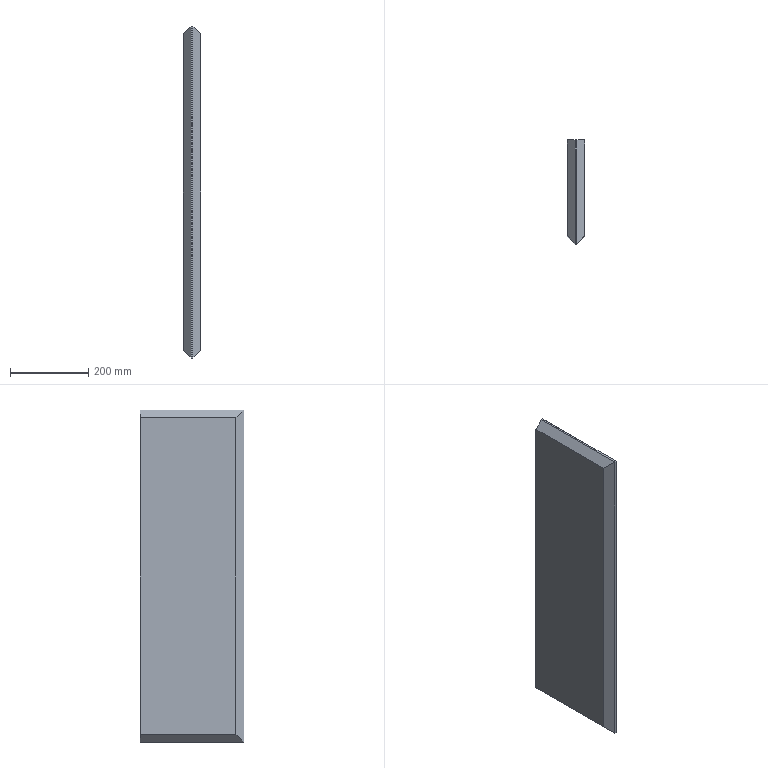Part | SolidWorks | features Chamfer 1, Extrusion 1 | 1 solid | 12 faces | box 45 x 265 x 850 mm | volume 9594917 mm3 | plane 12
STEP:
#1=CARTESIAN_POINT('',(2.5,132.5,425.));
#2=VERTEX_POINT('',#1);
#3=CARTESIAN_POINT('',(-2.5,132.5,425.));
#4=VERTEX_POINT('',#3);
#5=CARTESIAN_POINT('',(22.5,132.5,425.));
#6=DIRECTION('',(-1.,0.,0.));
#7=VECTOR('',#6,1000.);
#8=LINE('',#5,#7);
#9=EDGE_CURVE('',#2,#4,#8,.T.);
#10=ORIENTED_EDGE('',*,*,#9,.T.);
#11=CARTESIAN_POINT('',(-2.5,-132.5,425.));
#12=VERTEX_POINT('',#11);
#13=CARTESIAN_POINT('',(-2.5,-132.5,425.));
#14=DIRECTION('',(0.,-1.,0.));
#15=VECTOR('',#14,1000.);
#16=LINE('',#13,#15);
#17=EDGE_CURVE('',#4,#12,#16,.T.);
#18=ORIENTED_EDGE('',*,*,#17,.T.);
#19=CARTESIAN_POINT('',(2.5,-132.5,425.));
#20=VERTEX_POINT('',#19);
#21=CARTESIAN_POINT('',(22.5,-132.5,425.));
#22=DIRECTION('',(-1.,0.,0.));
#23=VECTOR('',#22,1000.);
#24=LINE('',#21,#23);
#25=EDGE_CURVE('',#20,#12,#24,.T.);
#26=ORIENTED_EDGE('',*,*,#25,.F.);
#27=CARTESIAN_POINT('',(2.5,132.5,425.));
#28=DIRECTION('',(0.,1.,0.));
#29=VECTOR('',#28,1000.);
#30=LINE('',#27,#29);
#31=EDGE_CURVE('',#20,#2,#30,.T.);
#32=ORIENTED_EDGE('',*,*,#31,.T.);
#33=EDGE_LOOP('',(#10,#18,#26,#32));
#34=FACE_OUTER_BOUND('',#33,.T.);
#35=CARTESIAN_POINT('',(22.5,-132.5,425.));
#36=DIRECTION('',(0.,0.,-1.));
#37=DIRECTION('',(-1.,0.,0.));
#38=AXIS2_PLACEMENT_3D('',#35,#36,#37);
#39=PLANE('',#38);
#40=ADVANCED_FACE('',(#34),#39,.F.);
#41=ORIENTED_EDGE('',*,*,#25,.T.);
#42=CARTESIAN_POINT('',(-2.5,-132.5,-425.));
#43=VERTEX_POINT('',#42);
#44=CARTESIAN_POINT('',(-2.5,-132.5,-425.));
#45=DIRECTION('',(0.,0.,-1.));
#46=VECTOR('',#45,1000.);
#47=LINE('',#44,#46);
#48=EDGE_CURVE('',#12,#43,#47,.T.);
#49=ORIENTED_EDGE('',*,*,#48,.T.);
#50=CARTESIAN_POINT('',(2.5,-132.5,-425.));
#51=VERTEX_POINT('',#50);
#52=CARTESIAN_POINT('',(22.5,-132.5,-425.));
#53=DIRECTION('',(-1.,0.,0.));
#54=VECTOR('',#53,1000.);
#55=LINE('',#52,#54);
#56=EDGE_CURVE('',#51,#43,#55,.T.);
#57=ORIENTED_EDGE('',*,*,#56,.F.);
#58=CARTESIAN_POINT('',(2.5,-132.5,425.));
#59=DIRECTION('',(0.,0.,1.));
#60=VECTOR('',#59,1000.);
#61=LINE('',#58,#60);
#62=EDGE_CURVE('',#51,#20,#61,.T.);
#63=ORIENTED_EDGE('',*,*,#62,.T.);
#64=EDGE_LOOP('',(#41,#49,#57,#63));
#65=FACE_OUTER_BOUND('',#64,.T.);
#66=CARTESIAN_POINT('',(22.5,-132.5,-425.));
#67=DIRECTION('',(0.,1.,0.));
#68=DIRECTION('',(0.,0.,1.));
#69=AXIS2_PLACEMENT_3D('',#66,#67,#68);
#70=PLANE('',#69);
#71=ADVANCED_FACE('',(#65),#70,.F.);
#72=ORIENTED_EDGE('',*,*,#56,.T.);
#73=CARTESIAN_POINT('',(-2.5,132.5,-425.));
#74=VERTEX_POINT('',#73);
#75=CARTESIAN_POINT('',(-2.5,-132.5,-425.));
#76=DIRECTION('',(0.,1.,0.));
#77=VECTOR('',#76,1000.);
#78=LINE('',#75,#77);
#79=EDGE_CURVE('',#43,#74,#78,.T.);
#80=ORIENTED_EDGE('',*,*,#79,.T.);
#81=CARTESIAN_POINT('',(2.5,132.5,-425.));
#82=VERTEX_POINT('',#81);
#83=CARTESIAN_POINT('',(22.5,132.5,-425.));
#84=DIRECTION('',(-1.,0.,0.));
#85=VECTOR('',#84,1000.);
#86=LINE('',#83,#85);
#87=EDGE_CURVE('',#82,#74,#86,.T.);
#88=ORIENTED_EDGE('',*,*,#87,.F.);
#89=CARTESIAN_POINT('',(2.5,-132.5,-425.));
#90=DIRECTION('',(0.,-1.,0.));
#91=VECTOR('',#90,1000.);
#92=LINE('',#89,#91);
#93=EDGE_CURVE('',#82,#51,#92,.T.);
#94=ORIENTED_EDGE('',*,*,#93,.T.);
#95=EDGE_LOOP('',(#72,#80,#88,#94));
#96=FACE_OUTER_BOUND('',#95,.T.);
#97=CARTESIAN_POINT('',(22.5,-132.5,-425.));
#98=DIRECTION('',(0.,0.,1.));
#99=DIRECTION('',(1.,0.,0.));
#100=AXIS2_PLACEMENT_3D('',#97,#98,#99);
#101=PLANE('',#100);
#102=ADVANCED_FACE('',(#96),#101,.F.);
#103=ORIENTED_EDGE('',*,*,#87,.T.);
#104=CARTESIAN_POINT('',(-22.5,132.5,-405.));
#105=VERTEX_POINT('',#104);
#106=CARTESIAN_POINT('',(-2.5,132.5,-425.));
#107=DIRECTION('',(-0.7071,0.,0.7071));
#108=VECTOR('',#107,1000.);
#109=LINE('',#106,#108);
#110=EDGE_CURVE('',#74,#105,#109,.T.);
#111=ORIENTED_EDGE('',*,*,#110,.T.);
#112=CARTESIAN_POINT('',(-22.5,132.5,405.));
#113=VERTEX_POINT('',#112);
#114=CARTESIAN_POINT('',(-22.5,132.5,-425.));
#115=DIRECTION('',(0.,0.,1.));
#116=VECTOR('',#115,1000.);
#117=LINE('',#114,#116);
#118=EDGE_CURVE('',#105,#113,#117,.T.);
#119=ORIENTED_EDGE('',*,*,#118,.T.);
#120=CARTESIAN_POINT('',(-2.5,132.5,425.));
#121=DIRECTION('',(0.7071,0.,0.7071));
#122=VECTOR('',#121,1000.);
#123=LINE('',#120,#122);
#124=EDGE_CURVE('',#113,#4,#123,.T.);
#125=ORIENTED_EDGE('',*,*,#124,.T.);
#126=ORIENTED_EDGE('',*,*,#9,.F.);
#127=CARTESIAN_POINT('',(22.5,132.5,405.));
#128=VERTEX_POINT('',#127);
#129=CARTESIAN_POINT('',(22.5,132.5,405.));
#130=DIRECTION('',(0.7071,0.,-0.7071));
#131=VECTOR('',#130,1000.);
#132=LINE('',#129,#131);
#133=EDGE_CURVE('',#2,#128,#132,.T.);
#134=ORIENTED_EDGE('',*,*,#133,.T.);
#135=CARTESIAN_POINT('',(22.5,132.5,-405.));
#136=VERTEX_POINT('',#135);
#137=CARTESIAN_POINT('',(22.5,132.5,-425.));
#138=DIRECTION('',(0.,0.,1.));
#139=VECTOR('',#138,1000.);
#140=LINE('',#137,#139);
#141=EDGE_CURVE('',#136,#128,#140,.T.);
#142=ORIENTED_EDGE('',*,*,#141,.F.);
#143=CARTESIAN_POINT('',(22.5,132.5,-405.));
#144=DIRECTION('',(-0.7071,0.,-0.7071));
#145=VECTOR('',#144,1000.);
#146=LINE('',#143,#145);
#147=EDGE_CURVE('',#136,#82,#146,.T.);
#148=ORIENTED_EDGE('',*,*,#147,.T.);
#149=EDGE_LOOP('',(#103,#111,#119,#125,#126,#134,#142,#148));
#150=FACE_OUTER_BOUND('',#149,.T.);
#151=CARTESIAN_POINT('',(22.5,132.5,-425.));
#152=DIRECTION('',(0.,-1.,0.));
#153=DIRECTION('',(0.,0.,-1.));
#154=AXIS2_PLACEMENT_3D('',#151,#152,#153);
#155=PLANE('',#154);
#156=ADVANCED_FACE('',(#150),#155,.F.);
#157=CARTESIAN_POINT('',(22.5,-112.5,405.));
#158=VERTEX_POINT('',#157);
#159=CARTESIAN_POINT('',(22.5,-112.5,-405.));
#160=VERTEX_POINT('',#159);
#161=CARTESIAN_POINT('',(22.5,-112.5,-425.));
#162=DIRECTION('',(0.,0.,-1.));
#163=VECTOR('',#162,1000.);
#164=LINE('',#161,#163);
#165=EDGE_CURVE('',#158,#160,#164,.T.);
#166=ORIENTED_EDGE('',*,*,#165,.T.);
#167=CARTESIAN_POINT('',(22.5,132.5,-405.));
#168=DIRECTION('',(0.,1.,0.));
#169=VECTOR('',#168,1000.);
#170=LINE('',#167,#169);
#171=EDGE_CURVE('',#160,#136,#170,.T.);
#172=ORIENTED_EDGE('',*,*,#171,.T.);
#173=ORIENTED_EDGE('',*,*,#141,.T.);
#174=CARTESIAN_POINT('',(22.5,-132.5,405.));
#175=DIRECTION('',(0.,-1.,0.));
#176=VECTOR('',#175,1000.);
#177=LINE('',#174,#176);
#178=EDGE_CURVE('',#128,#158,#177,.T.);
#179=ORIENTED_EDGE('',*,*,#178,.T.);
#180=EDGE_LOOP('',(#166,#172,#173,#179));
#181=FACE_OUTER_BOUND('',#180,.T.);
#182=CARTESIAN_POINT('',(22.5,0.,0.));
#183=DIRECTION('',(1.,0.,0.));
#184=DIRECTION('',(0.,0.,-1.));
#185=AXIS2_PLACEMENT_3D('',#182,#183,#184);
#186=PLANE('',#185);
#187=ADVANCED_FACE('',(#181),#186,.T.);
#188=ORIENTED_EDGE('',*,*,#118,.F.);
#189=CARTESIAN_POINT('',(-22.5,-112.5,-405.));
#190=VERTEX_POINT('',#189);
#191=CARTESIAN_POINT('',(-22.5,0.,-405.));
#192=DIRECTION('',(0.,-1.,0.));
#193=VECTOR('',#192,1000.);
#194=LINE('',#191,#193);
#195=EDGE_CURVE('',#105,#190,#194,.T.);
#196=ORIENTED_EDGE('',*,*,#195,.T.);
#197=CARTESIAN_POINT('',(-22.5,-112.5,405.));
#198=VERTEX_POINT('',#197);
#199=CARTESIAN_POINT('',(-22.5,-112.5,0.));
#200=DIRECTION('',(0.,0.,1.));
#201=VECTOR('',#200,1000.);
#202=LINE('',#199,#201);
#203=EDGE_CURVE('',#190,#198,#202,.T.);
#204=ORIENTED_EDGE('',*,*,#203,.T.);
#205=CARTESIAN_POINT('',(-22.5,0.,405.));
#206=DIRECTION('',(0.,1.,0.));
#207=VECTOR('',#206,1000.);
#208=LINE('',#205,#207);
#209=EDGE_CURVE('',#198,#113,#208,.T.);
#210=ORIENTED_EDGE('',*,*,#209,.T.);
#211=EDGE_LOOP('',(#188,#196,#204,#210));
#212=FACE_OUTER_BOUND('',#211,.T.);
#213=CARTESIAN_POINT('',(-22.5,0.,0.));
#214=DIRECTION('',(1.,0.,0.));
#215=DIRECTION('',(0.,0.,-1.));
#216=AXIS2_PLACEMENT_3D('',#213,#214,#215);
#217=PLANE('',#216);
#218=ADVANCED_FACE('',(#212),#217,.F.);
#219=ORIENTED_EDGE('',*,*,#124,.F.);
#220=ORIENTED_EDGE('',*,*,#209,.F.);
#221=CARTESIAN_POINT('',(-2.5,-132.5,425.));
#222=DIRECTION('',(-0.5774,0.5774,-0.5774));
#223=VECTOR('',#222,1000.);
#224=LINE('',#221,#223);
#225=EDGE_CURVE('',#12,#198,#224,.T.);
#226=ORIENTED_EDGE('',*,*,#225,.F.);
#227=ORIENTED_EDGE('',*,*,#17,.F.);
#228=EDGE_LOOP('',(#219,#220,#226,#227));
#229=FACE_OUTER_BOUND('',#228,.T.);
#230=CARTESIAN_POINT('',(-2.5,-132.5,425.));
#231=DIRECTION('',(0.7071,0.,-0.7071));
#232=DIRECTION('',(0.,-1.,0.));
#233=AXIS2_PLACEMENT_3D('',#230,#231,#232);
#234=PLANE('',#233);
#235=ADVANCED_FACE('',(#229),#234,.F.);
#236=ORIENTED_EDGE('',*,*,#225,.T.);
#237=ORIENTED_EDGE('',*,*,#203,.F.);
#238=CARTESIAN_POINT('',(-2.5,-132.5,-425.));
#239=DIRECTION('',(-0.5774,0.5774,0.5774));
#240=VECTOR('',#239,1000.);
#241=LINE('',#238,#240);
#242=EDGE_CURVE('',#43,#190,#241,.T.);
#243=ORIENTED_EDGE('',*,*,#242,.F.);
#244=ORIENTED_EDGE('',*,*,#48,.F.);
#245=EDGE_LOOP('',(#236,#237,#243,#244));
#246=FACE_OUTER_BOUND('',#245,.T.);
#247=CARTESIAN_POINT('',(-2.5,-132.5,-425.));
#248=DIRECTION('',(0.7071,0.7071,0.));
#249=DIRECTION('',(0.,0.,-1.));
#250=AXIS2_PLACEMENT_3D('',#247,#248,#249);
#251=PLANE('',#250);
#252=ADVANCED_FACE('',(#246),#251,.F.);
#253=ORIENTED_EDGE('',*,*,#242,.T.);
#254=ORIENTED_EDGE('',*,*,#195,.F.);
#255=ORIENTED_EDGE('',*,*,#110,.F.);
#256=ORIENTED_EDGE('',*,*,#79,.F.);
#257=EDGE_LOOP('',(#253,#254,#255,#256));
#258=FACE_OUTER_BOUND('',#257,.T.);
#259=CARTESIAN_POINT('',(-2.5,-132.5,-425.));
#260=DIRECTION('',(0.7071,0.,0.7071));
#261=DIRECTION('',(0.,1.,0.));
#262=AXIS2_PLACEMENT_3D('',#259,#260,#261);
#263=PLANE('',#262);
#264=ADVANCED_FACE('',(#258),#263,.F.);
#265=ORIENTED_EDGE('',*,*,#133,.F.);
#266=ORIENTED_EDGE('',*,*,#31,.F.);
#267=CARTESIAN_POINT('',(60.,-75.,367.5));
#268=DIRECTION('',(-0.5774,-0.5774,0.5774));
#269=VECTOR('',#268,1000.);
#270=LINE('',#267,#269);
#271=EDGE_CURVE('',#158,#20,#270,.T.);
#272=ORIENTED_EDGE('',*,*,#271,.F.);
#273=ORIENTED_EDGE('',*,*,#178,.F.);
#274=EDGE_LOOP('',(#265,#266,#272,#273));
#275=FACE_OUTER_BOUND('',#274,.T.);
#276=CARTESIAN_POINT('',(22.5,0.,405.));
#277=DIRECTION('',(0.7071,0.,0.7071));
#278=DIRECTION('',(0.,1.,0.));
#279=AXIS2_PLACEMENT_3D('',#276,#277,#278);
#280=PLANE('',#279);
#281=ADVANCED_FACE('',(#275),#280,.T.);
#282=ORIENTED_EDGE('',*,*,#271,.T.);
#283=ORIENTED_EDGE('',*,*,#62,.F.);
#284=CARTESIAN_POINT('',(157.5,22.5,-270.));
#285=DIRECTION('',(-0.5774,-0.5774,-0.5774));
#286=VECTOR('',#285,1000.);
#287=LINE('',#284,#286);
#288=EDGE_CURVE('',#160,#51,#287,.T.);
#289=ORIENTED_EDGE('',*,*,#288,.F.);
#290=ORIENTED_EDGE('',*,*,#165,.F.);
#291=EDGE_LOOP('',(#282,#283,#289,#290));
#292=FACE_OUTER_BOUND('',#291,.T.);
#293=CARTESIAN_POINT('',(22.5,-112.5,0.));
#294=DIRECTION('',(0.7071,-0.7071,0.));
#295=DIRECTION('',(0.,0.,1.));
#296=AXIS2_PLACEMENT_3D('',#293,#294,#295);
#297=PLANE('',#296);
#298=ADVANCED_FACE('',(#292),#297,.T.);
#299=ORIENTED_EDGE('',*,*,#288,.T.);
#300=ORIENTED_EDGE('',*,*,#93,.F.);
#301=ORIENTED_EDGE('',*,*,#147,.F.);
#302=ORIENTED_EDGE('',*,*,#171,.F.);
#303=EDGE_LOOP('',(#299,#300,#301,#302));
#304=FACE_OUTER_BOUND('',#303,.T.);
#305=CARTESIAN_POINT('',(22.5,0.,-405.));
#306=DIRECTION('',(0.7071,0.,-0.7071));
#307=DIRECTION('',(0.,-1.,0.));
#308=AXIS2_PLACEMENT_3D('',#305,#306,#307);
#309=PLANE('',#308);
#310=ADVANCED_FACE('',(#304),#309,.T.);
#311=CLOSED_SHELL('',(#40,#71,#102,#156,#187,#218,#235,#252,#264,#281,#298,#310));
#312=MANIFOLD_SOLID_BREP('',#311);
#313=CARTESIAN_POINT('',(0.,0.,0.));
#314=DIRECTION('',(0.,0.,1.));
#315=DIRECTION('',(1.,0.,0.));
#316=AXIS2_PLACEMENT_3D('',#313,#314,#315);
#317=(LENGTH_UNIT()NAMED_UNIT(*)SI_UNIT(.MILLI.,.METRE.));
#318=UNCERTAINTY_MEASURE_WITH_UNIT(LENGTH_MEASURE(0.00001),#317,'','');
#319=(NAMED_UNIT(*)PLANE_ANGLE_UNIT()SI_UNIT($,.RADIAN.));
#320=(NAMED_UNIT(*)SI_UNIT($,.STERADIAN.)SOLID_ANGLE_UNIT());
#321=(GEOMETRIC_REPRESENTATION_CONTEXT(3)GLOBAL_UNCERTAINTY_ASSIGNED_CONTEXT((#318))GLOBAL_UNIT_ASSIGNED_CONTEXT((#317,#319,#320))REPRESENTATION_CONTEXT('',''));
#322=ADVANCED_BREP_SHAPE_REPRESENTATION('',(#312,#316),#321);